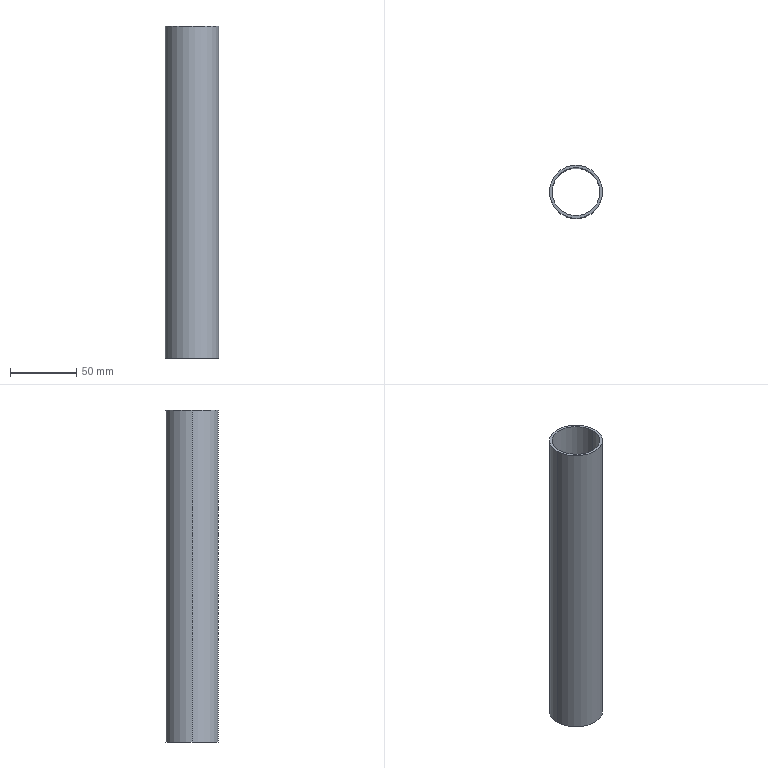Part | SolidWorks | features Extrusion 1 | 1 solid | 6 faces | box 40 x 40 x 250 mm | volume 59690 mm3 | cylinder 4 | plane 2 | commonest cylinder face diameters 36 x2 40 x2
STEP:
#1=CARTESIAN_POINT('',(-18.,0.,250.));
#2=VERTEX_POINT('',#1);
#3=CARTESIAN_POINT('',(18.,0.,250.));
#4=VERTEX_POINT('',#3);
#5=CARTESIAN_POINT('',(0.,0.,250.));
#6=DIRECTION('',(0.,0.,1.));
#7=DIRECTION('',(1.,0.,0.));
#8=AXIS2_PLACEMENT_3D('',#5,#6,#7);
#9=CIRCLE('',#8,18.);
#10=EDGE_CURVE('',#2,#4,#9,.T.);
#11=ORIENTED_EDGE('',*,*,#10,.T.);
#12=CARTESIAN_POINT('',(18.,0.,0.));
#13=VERTEX_POINT('',#12);
#14=CARTESIAN_POINT('',(18.,0.,250.));
#15=DIRECTION('',(0.,0.,-1.));
#16=VECTOR('',#15,1000.);
#17=LINE('',#14,#16);
#18=EDGE_CURVE('',#4,#13,#17,.T.);
#19=ORIENTED_EDGE('',*,*,#18,.T.);
#20=CARTESIAN_POINT('',(-18.,0.,0.));
#21=VERTEX_POINT('',#20);
#22=CARTESIAN_POINT('',(0.,0.,0.));
#23=DIRECTION('',(0.,0.,1.));
#24=DIRECTION('',(1.,0.,0.));
#25=AXIS2_PLACEMENT_3D('',#22,#23,#24);
#26=CIRCLE('',#25,18.);
#27=EDGE_CURVE('',#21,#13,#26,.T.);
#28=ORIENTED_EDGE('',*,*,#27,.F.);
#29=CARTESIAN_POINT('',(-18.,0.,250.));
#30=DIRECTION('',(0.,0.,-1.));
#31=VECTOR('',#30,1000.);
#32=LINE('',#29,#31);
#33=EDGE_CURVE('',#2,#21,#32,.T.);
#34=ORIENTED_EDGE('',*,*,#33,.F.);
#35=EDGE_LOOP('',(#11,#19,#28,#34));
#36=FACE_OUTER_BOUND('',#35,.T.);
#37=CARTESIAN_POINT('',(0.,0.,250.));
#38=DIRECTION('',(0.,0.,-1.));
#39=DIRECTION('',(-1.,0.,0.));
#40=AXIS2_PLACEMENT_3D('',#37,#38,#39);
#41=CYLINDRICAL_SURFACE('',#40,18.);
#42=ADVANCED_FACE('',(#36),#41,.F.);
#43=CARTESIAN_POINT('',(20.,0.,250.));
#44=VERTEX_POINT('',#43);
#45=CARTESIAN_POINT('',(-20.,0.,250.));
#46=VERTEX_POINT('',#45);
#47=CARTESIAN_POINT('',(0.,0.,250.));
#48=DIRECTION('',(0.,0.,1.));
#49=DIRECTION('',(1.,0.,0.));
#50=AXIS2_PLACEMENT_3D('',#47,#48,#49);
#51=CIRCLE('',#50,20.);
#52=EDGE_CURVE('',#44,#46,#51,.T.);
#53=ORIENTED_EDGE('',*,*,#52,.F.);
#54=CARTESIAN_POINT('',(20.,0.,0.));
#55=VERTEX_POINT('',#54);
#56=CARTESIAN_POINT('',(20.,0.,250.));
#57=DIRECTION('',(0.,0.,-1.));
#58=VECTOR('',#57,1000.);
#59=LINE('',#56,#58);
#60=EDGE_CURVE('',#44,#55,#59,.T.);
#61=ORIENTED_EDGE('',*,*,#60,.T.);
#62=CARTESIAN_POINT('',(-20.,0.,0.));
#63=VERTEX_POINT('',#62);
#64=CARTESIAN_POINT('',(0.,0.,0.));
#65=DIRECTION('',(0.,0.,1.));
#66=DIRECTION('',(1.,0.,0.));
#67=AXIS2_PLACEMENT_3D('',#64,#65,#66);
#68=CIRCLE('',#67,20.);
#69=EDGE_CURVE('',#55,#63,#68,.T.);
#70=ORIENTED_EDGE('',*,*,#69,.T.);
#71=CARTESIAN_POINT('',(-20.,0.,250.));
#72=DIRECTION('',(0.,0.,-1.));
#73=VECTOR('',#72,1000.);
#74=LINE('',#71,#73);
#75=EDGE_CURVE('',#46,#63,#74,.T.);
#76=ORIENTED_EDGE('',*,*,#75,.F.);
#77=EDGE_LOOP('',(#53,#61,#70,#76));
#78=FACE_OUTER_BOUND('',#77,.T.);
#79=CARTESIAN_POINT('',(0.,0.,250.));
#80=DIRECTION('',(0.,0.,-1.));
#81=DIRECTION('',(-1.,0.,0.));
#82=AXIS2_PLACEMENT_3D('',#79,#80,#81);
#83=CYLINDRICAL_SURFACE('',#82,20.);
#84=ADVANCED_FACE('',(#78),#83,.T.);
#85=CARTESIAN_POINT('',(0.,0.,250.));
#86=DIRECTION('',(0.,0.,1.));
#87=DIRECTION('',(1.,0.,0.));
#88=AXIS2_PLACEMENT_3D('',#85,#86,#87);
#89=CIRCLE('',#88,20.);
#90=EDGE_CURVE('',#46,#44,#89,.T.);
#91=ORIENTED_EDGE('',*,*,#90,.T.);
#92=ORIENTED_EDGE('',*,*,#52,.T.);
#93=EDGE_LOOP('',(#91,#92));
#94=FACE_OUTER_BOUND('',#93,.T.);
#95=ORIENTED_EDGE('',*,*,#10,.F.);
#96=CARTESIAN_POINT('',(0.,0.,250.));
#97=DIRECTION('',(0.,0.,1.));
#98=DIRECTION('',(1.,0.,0.));
#99=AXIS2_PLACEMENT_3D('',#96,#97,#98);
#100=CIRCLE('',#99,18.);
#101=EDGE_CURVE('',#4,#2,#100,.T.);
#102=ORIENTED_EDGE('',*,*,#101,.F.);
#103=EDGE_LOOP('',(#95,#102));
#104=FACE_BOUND('',#103,.T.);
#105=CARTESIAN_POINT('',(0.,0.,250.));
#106=DIRECTION('',(0.,0.,1.));
#107=DIRECTION('',(1.,0.,0.));
#108=AXIS2_PLACEMENT_3D('',#105,#106,#107);
#109=PLANE('',#108);
#110=ADVANCED_FACE('',(#94,#104),#109,.T.);
#111=CARTESIAN_POINT('',(0.,0.,0.));
#112=DIRECTION('',(0.,0.,1.));
#113=DIRECTION('',(1.,0.,0.));
#114=AXIS2_PLACEMENT_3D('',#111,#112,#113);
#115=CIRCLE('',#114,20.);
#116=EDGE_CURVE('',#63,#55,#115,.T.);
#117=ORIENTED_EDGE('',*,*,#116,.F.);
#118=ORIENTED_EDGE('',*,*,#69,.F.);
#119=EDGE_LOOP('',(#117,#118));
#120=FACE_OUTER_BOUND('',#119,.T.);
#121=ORIENTED_EDGE('',*,*,#27,.T.);
#122=CARTESIAN_POINT('',(0.,0.,0.));
#123=DIRECTION('',(0.,0.,1.));
#124=DIRECTION('',(1.,0.,0.));
#125=AXIS2_PLACEMENT_3D('',#122,#123,#124);
#126=CIRCLE('',#125,18.);
#127=EDGE_CURVE('',#13,#21,#126,.T.);
#128=ORIENTED_EDGE('',*,*,#127,.T.);
#129=EDGE_LOOP('',(#121,#128));
#130=FACE_BOUND('',#129,.T.);
#131=CARTESIAN_POINT('',(0.,0.,0.));
#132=DIRECTION('',(0.,0.,1.));
#133=DIRECTION('',(1.,0.,0.));
#134=AXIS2_PLACEMENT_3D('',#131,#132,#133);
#135=PLANE('',#134);
#136=ADVANCED_FACE('',(#120,#130),#135,.F.);
#137=ORIENTED_EDGE('',*,*,#60,.F.);
#138=ORIENTED_EDGE('',*,*,#90,.F.);
#139=ORIENTED_EDGE('',*,*,#75,.T.);
#140=ORIENTED_EDGE('',*,*,#116,.T.);
#141=EDGE_LOOP('',(#137,#138,#139,#140));
#142=FACE_OUTER_BOUND('',#141,.T.);
#143=CARTESIAN_POINT('',(0.,0.,250.));
#144=DIRECTION('',(0.,0.,-1.));
#145=DIRECTION('',(-1.,0.,0.));
#146=AXIS2_PLACEMENT_3D('',#143,#144,#145);
#147=CYLINDRICAL_SURFACE('',#146,20.);
#148=ADVANCED_FACE('',(#142),#147,.T.);
#149=ORIENTED_EDGE('',*,*,#18,.F.);
#150=ORIENTED_EDGE('',*,*,#101,.T.);
#151=ORIENTED_EDGE('',*,*,#33,.T.);
#152=ORIENTED_EDGE('',*,*,#127,.F.);
#153=EDGE_LOOP('',(#149,#150,#151,#152));
#154=FACE_OUTER_BOUND('',#153,.T.);
#155=CARTESIAN_POINT('',(0.,0.,250.));
#156=DIRECTION('',(0.,0.,-1.));
#157=DIRECTION('',(-1.,0.,0.));
#158=AXIS2_PLACEMENT_3D('',#155,#156,#157);
#159=CYLINDRICAL_SURFACE('',#158,18.);
#160=ADVANCED_FACE('',(#154),#159,.F.);
#161=CLOSED_SHELL('',(#42,#84,#110,#136,#148,#160));
#162=MANIFOLD_SOLID_BREP('',#161);
#163=CARTESIAN_POINT('',(0.,0.,0.));
#164=DIRECTION('',(0.,0.,1.));
#165=DIRECTION('',(1.,0.,0.));
#166=AXIS2_PLACEMENT_3D('',#163,#164,#165);
#167=(LENGTH_UNIT()NAMED_UNIT(*)SI_UNIT(.MILLI.,.METRE.));
#168=UNCERTAINTY_MEASURE_WITH_UNIT(LENGTH_MEASURE(0.00001),#167,'','');
#169=(NAMED_UNIT(*)PLANE_ANGLE_UNIT()SI_UNIT($,.RADIAN.));
#170=(NAMED_UNIT(*)SI_UNIT($,.STERADIAN.)SOLID_ANGLE_UNIT());
#171=(GEOMETRIC_REPRESENTATION_CONTEXT(3)GLOBAL_UNCERTAINTY_ASSIGNED_CONTEXT((#168))GLOBAL_UNIT_ASSIGNED_CONTEXT((#167,#169,#170))REPRESENTATION_CONTEXT('',''));
#172=ADVANCED_BREP_SHAPE_REPRESENTATION('',(#162,#166),#171);